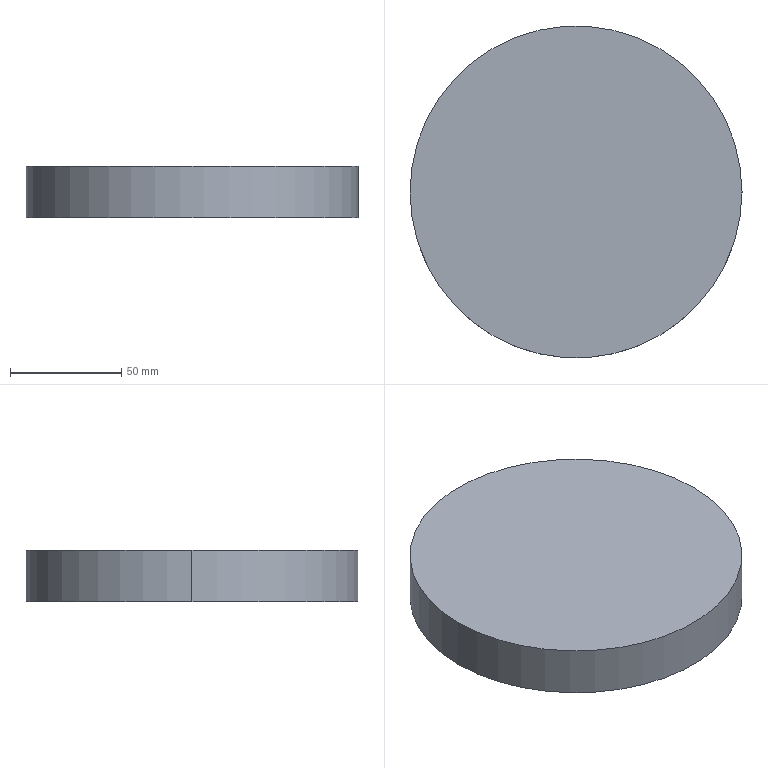Part | SolidWorks | features Extrusion 1 | 1 solid | 4 faces | box 149 x 149 x 23 mm | volume 401042 mm3 | cylinder 2 | plane 2 | commonest cylinder face diameters 149 x2
STEP:
#1=CARTESIAN_POINT('',(74.5,0.,23.));
#2=VERTEX_POINT('',#1);
#3=CARTESIAN_POINT('',(-74.5,0.,23.));
#4=VERTEX_POINT('',#3);
#5=CARTESIAN_POINT('',(0.,0.,23.));
#6=DIRECTION('',(0.,0.,1.));
#7=DIRECTION('',(1.,0.,0.));
#8=AXIS2_PLACEMENT_3D('',#5,#6,#7);
#9=CIRCLE('',#8,74.5);
#10=EDGE_CURVE('',#2,#4,#9,.T.);
#11=ORIENTED_EDGE('',*,*,#10,.F.);
#12=CARTESIAN_POINT('',(74.5,0.,0.));
#13=VERTEX_POINT('',#12);
#14=CARTESIAN_POINT('',(74.5,0.,23.));
#15=DIRECTION('',(0.,0.,-1.));
#16=VECTOR('',#15,1000.);
#17=LINE('',#14,#16);
#18=EDGE_CURVE('',#2,#13,#17,.T.);
#19=ORIENTED_EDGE('',*,*,#18,.T.);
#20=CARTESIAN_POINT('',(-74.5,0.,0.));
#21=VERTEX_POINT('',#20);
#22=CARTESIAN_POINT('',(0.,0.,0.));
#23=DIRECTION('',(0.,0.,1.));
#24=DIRECTION('',(1.,0.,0.));
#25=AXIS2_PLACEMENT_3D('',#22,#23,#24);
#26=CIRCLE('',#25,74.5);
#27=EDGE_CURVE('',#13,#21,#26,.T.);
#28=ORIENTED_EDGE('',*,*,#27,.T.);
#29=CARTESIAN_POINT('',(-74.5,0.,23.));
#30=DIRECTION('',(0.,0.,-1.));
#31=VECTOR('',#30,1000.);
#32=LINE('',#29,#31);
#33=EDGE_CURVE('',#4,#21,#32,.T.);
#34=ORIENTED_EDGE('',*,*,#33,.F.);
#35=EDGE_LOOP('',(#11,#19,#28,#34));
#36=FACE_OUTER_BOUND('',#35,.T.);
#37=CARTESIAN_POINT('',(0.,0.,23.));
#38=DIRECTION('',(0.,0.,-1.));
#39=DIRECTION('',(-1.,0.,0.));
#40=AXIS2_PLACEMENT_3D('',#37,#38,#39);
#41=CYLINDRICAL_SURFACE('',#40,74.5);
#42=ADVANCED_FACE('',(#36),#41,.T.);
#43=ORIENTED_EDGE('',*,*,#18,.F.);
#44=CARTESIAN_POINT('',(0.,0.,23.));
#45=DIRECTION('',(0.,0.,1.));
#46=DIRECTION('',(1.,0.,0.));
#47=AXIS2_PLACEMENT_3D('',#44,#45,#46);
#48=CIRCLE('',#47,74.5);
#49=EDGE_CURVE('',#4,#2,#48,.T.);
#50=ORIENTED_EDGE('',*,*,#49,.F.);
#51=ORIENTED_EDGE('',*,*,#33,.T.);
#52=CARTESIAN_POINT('',(0.,0.,0.));
#53=DIRECTION('',(0.,0.,1.));
#54=DIRECTION('',(1.,0.,0.));
#55=AXIS2_PLACEMENT_3D('',#52,#53,#54);
#56=CIRCLE('',#55,74.5);
#57=EDGE_CURVE('',#21,#13,#56,.T.);
#58=ORIENTED_EDGE('',*,*,#57,.T.);
#59=EDGE_LOOP('',(#43,#50,#51,#58));
#60=FACE_OUTER_BOUND('',#59,.T.);
#61=CARTESIAN_POINT('',(0.,0.,23.));
#62=DIRECTION('',(0.,0.,-1.));
#63=DIRECTION('',(-1.,0.,0.));
#64=AXIS2_PLACEMENT_3D('',#61,#62,#63);
#65=CYLINDRICAL_SURFACE('',#64,74.5);
#66=ADVANCED_FACE('',(#60),#65,.T.);
#67=ORIENTED_EDGE('',*,*,#49,.T.);
#68=ORIENTED_EDGE('',*,*,#10,.T.);
#69=EDGE_LOOP('',(#67,#68));
#70=FACE_OUTER_BOUND('',#69,.T.);
#71=CARTESIAN_POINT('',(0.,0.,23.));
#72=DIRECTION('',(0.,0.,1.));
#73=DIRECTION('',(1.,0.,0.));
#74=AXIS2_PLACEMENT_3D('',#71,#72,#73);
#75=PLANE('',#74);
#76=ADVANCED_FACE('',(#70),#75,.T.);
#77=ORIENTED_EDGE('',*,*,#57,.F.);
#78=ORIENTED_EDGE('',*,*,#27,.F.);
#79=EDGE_LOOP('',(#77,#78));
#80=FACE_OUTER_BOUND('',#79,.T.);
#81=CARTESIAN_POINT('',(0.,0.,0.));
#82=DIRECTION('',(0.,0.,1.));
#83=DIRECTION('',(1.,0.,0.));
#84=AXIS2_PLACEMENT_3D('',#81,#82,#83);
#85=PLANE('',#84);
#86=ADVANCED_FACE('',(#80),#85,.F.);
#87=CLOSED_SHELL('',(#42,#66,#76,#86));
#88=MANIFOLD_SOLID_BREP('',#87);
#89=CARTESIAN_POINT('',(0.,0.,0.));
#90=DIRECTION('',(0.,0.,1.));
#91=DIRECTION('',(1.,0.,0.));
#92=AXIS2_PLACEMENT_3D('',#89,#90,#91);
#93=(LENGTH_UNIT()NAMED_UNIT(*)SI_UNIT(.MILLI.,.METRE.));
#94=UNCERTAINTY_MEASURE_WITH_UNIT(LENGTH_MEASURE(0.00001),#93,'','');
#95=(NAMED_UNIT(*)PLANE_ANGLE_UNIT()SI_UNIT($,.RADIAN.));
#96=(NAMED_UNIT(*)SI_UNIT($,.STERADIAN.)SOLID_ANGLE_UNIT());
#97=(GEOMETRIC_REPRESENTATION_CONTEXT(3)GLOBAL_UNCERTAINTY_ASSIGNED_CONTEXT((#94))GLOBAL_UNIT_ASSIGNED_CONTEXT((#93,#95,#96))REPRESENTATION_CONTEXT('',''));
#98=ADVANCED_BREP_SHAPE_REPRESENTATION('',(#88,#92),#97);